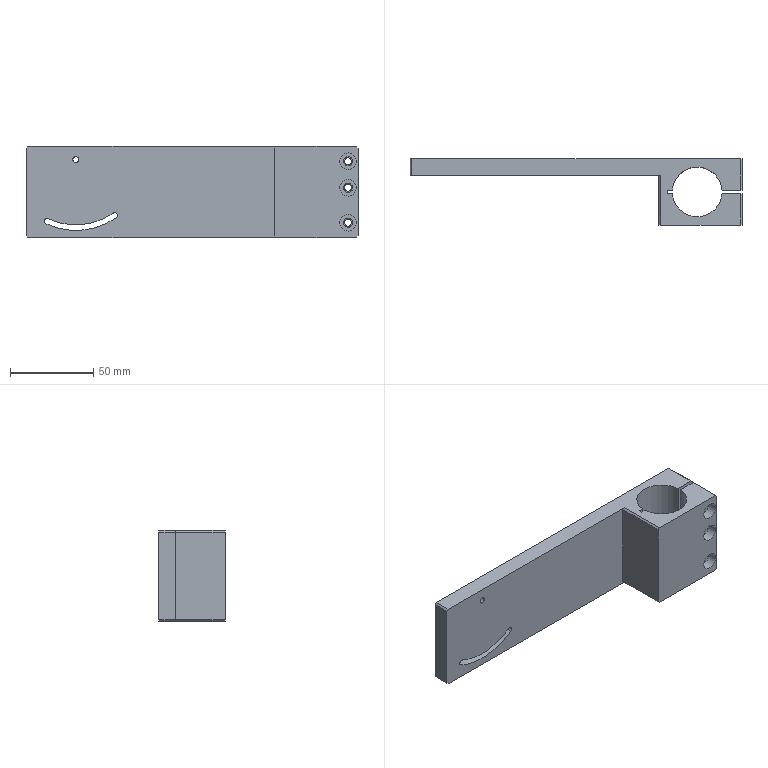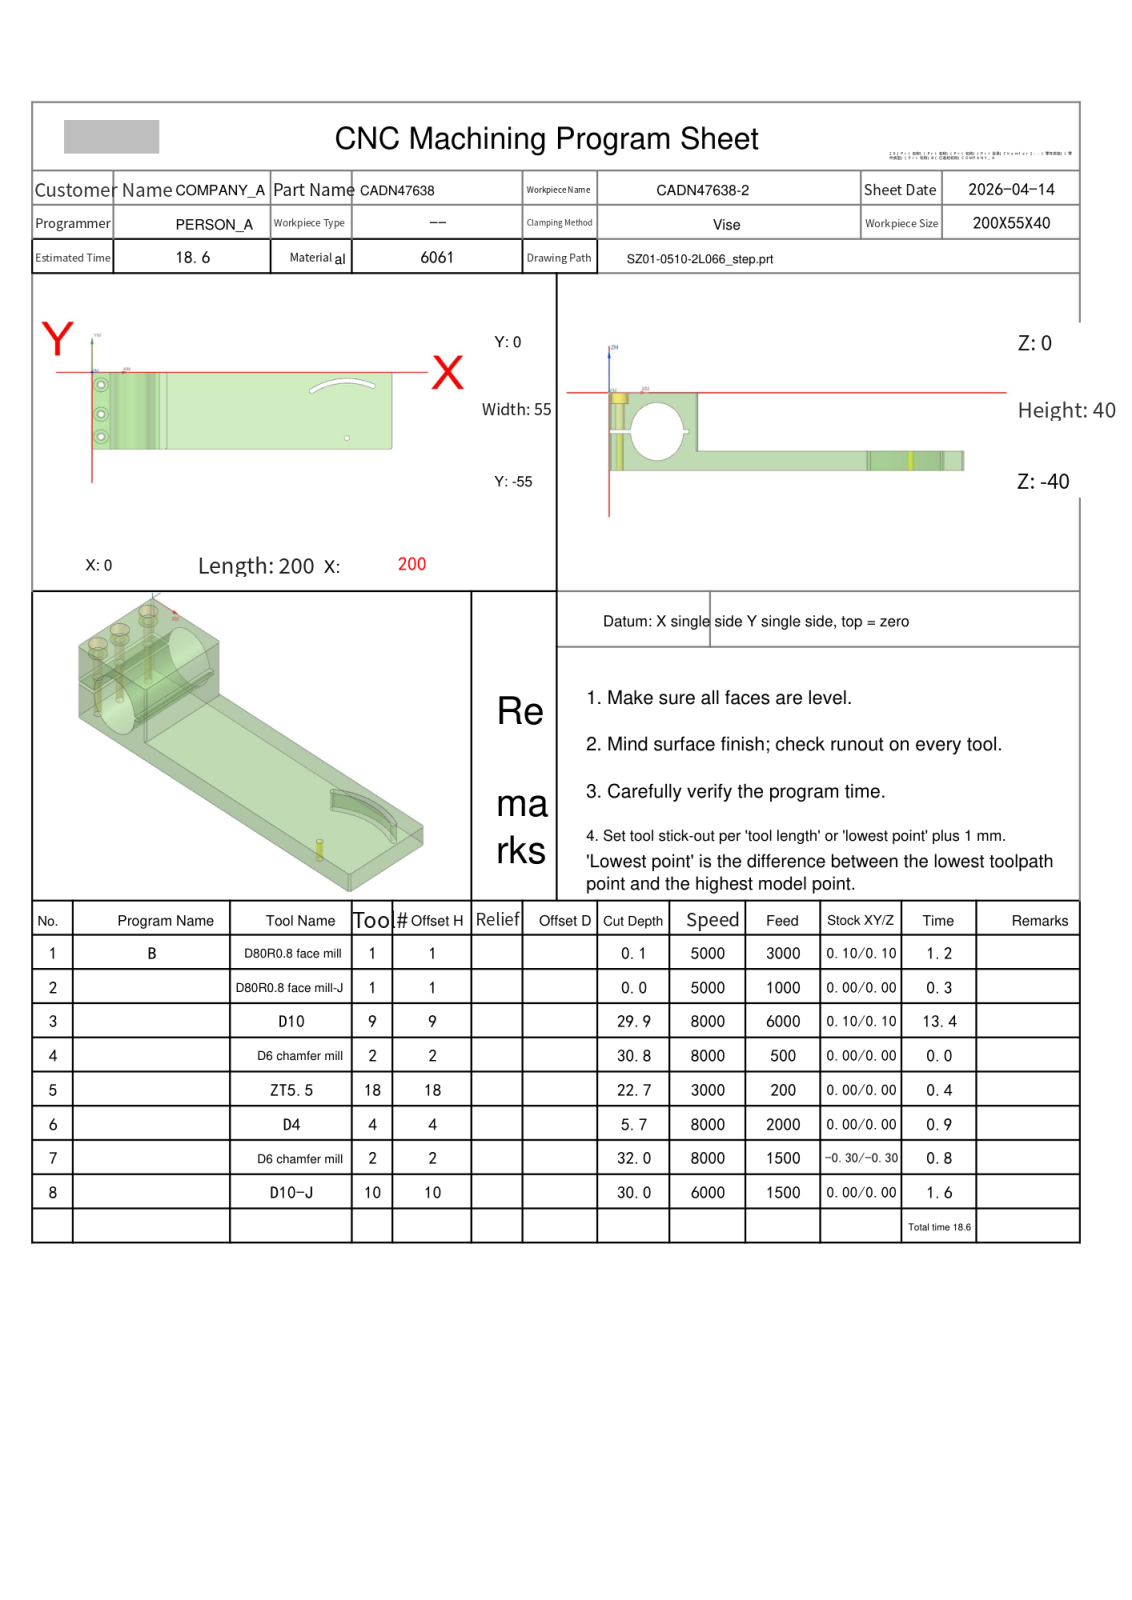NC program | NX | posted by the shop | part box 200 x 40 x 55 mm
Lines 7724 to 8619 of 8619:
N4 T02 M06
(D6 chamfer mill D=6. R=0. H=02 ce=0.00 di=0.10)
(MAX_Z=20. MIN_Z=-30.8 Time=0.04M)
G00 G90 G54 X170. Y-47. M03 S8000
G43 H02 Z20.
M08
G98 G81 X170. Y-47. Z-30.8 R-29. F500.
X6. Y-46. Z-.8 R1.
Y-30.
Y-9.
G80
G00 Z20.
G91 G28 Z0.0
M05
M09
G91 G28 Z0.0
M01
N5 T18 M06
(ZT5.5 D=5.5 DR_a=118 H=18)
(MAX_Z=20. MIN_Z=-22.65 Time=0.36M)
G00 G90 G54 X6. Y-46. M03 S3000
G43 H18 Z20.
M08
G98 G83 X6. Y-46. Z-22.652 R1. F200. Q2.
Y-30.
Y-9.
G80
G00 Z20.
G91 G28 Z0.0
M05
M09
G91 G28 Z0.0
M01
N6 T04 M06
(D4  D=4. R=0. H=04 ce=0.10 di=0.08)
(D.N=04 MAX_Z=20. MIN_Z=-5.7 Time=0.92M)
G00 G90 G54 X4.558 Y-32.526 M03 S8000
G43 H04 Z20.
M08
Z.8
G01 X4.688 Y-32.62 Z.792 F2000.
X5.582 Y-32.9 Z.743
X6.418 Z.699
X7.312 Y-32.62 Z.65
X8.072 Y-32.072 Z.601
X8.62 Y-31.312 Z.551
X8.9 Y-30.418 Z.502
Y-29.582 Z.458
X8.62 Y-28.688 Z.409
X8.072 Y-27.928 Z.36
X7.312 Y-27.38 Z.311
X6.418 Y-27.1 Z.262
X5.582 Z.218
X4.688 Y-27.38 Z.169
X3.928 Y-27.928 Z.12
X3.38 Y-28.688 Z.071
X3.1 Y-29.582 Z.022
Y-30. Z0.0
G03 X6. Y-32.9 Z-.074 I2.9 J0.0
X8.9 Y-30. Z-.148 I0.0 J2.9
X6. Y-27.1 Z-.223 I-2.9 J0.0
X3.1 Y-30. Z-.297 I0.0 J-2.9
X6. Y-32.9 Z-.371 I2.9 J0.0
X8.9 Y-30. Z-.445 I0.0 J2.9
X6. Y-27.1 Z-.519 I-2.9 J0.0
X3.1 Y-30. Z-.594 I0.0 J-2.9
X6. Y-32.9 Z-.668 I2.9 J0.0
X8.9 Y-30. Z-.742 I0.0 J2.9
X6. Y-27.1 Z-.816 I-2.9 J0.0
X3.1 Y-30. Z-.891 I0.0 J-2.9
X6. Y-32.9 Z-.965 I2.9 J0.0
X8.9 Y-30. Z-1.039 I0.0 J2.9
X6. Y-27.1 Z-1.113 I-2.9 J0.0
X3.1 Y-30. Z-1.187 I0.0 J-2.9
X6. Y-32.9 Z-1.262 I2.9 J0.0
X8.9 Y-30. Z-1.336 I0.0 J2.9
X6. Y-27.1 Z-1.41 I-2.9 J0.0
X3.1 Y-30. Z-1.484 I0.0 J-2.9
X6. Y-32.9 Z-1.558 I2.9 J0.0
X8.9 Y-30. Z-1.633 I0.0 J2.9
X6. Y-27.1 Z-1.707 I-2.9 J0.0
X3.1 Y-30. Z-1.781 I0.0 J-2.9
X6. Y-32.9 Z-1.855 I2.9 J0.0
X8.9 Y-30. Z-1.929 I0.0 J2.9
X6. Y-27.1 Z-2.004 I-2.9 J0.0
X3.1 Y-30. Z-2.078 I0.0 J-2.9
X6. Y-32.9 Z-2.152 I2.9 J0.0
X8.9 Y-30. Z-2.226 I0.0 J2.9
X6. Y-27.1 Z-2.301 I-2.9 J0.0
X3.1 Y-30. Z-2.375 I0.0 J-2.9
X6. Y-32.9 Z-2.449 I2.9 J0.0
X8.9 Y-30. Z-2.523 I0.0 J2.9
X6. Y-27.1 Z-2.597 I-2.9 J0.0
X3.1 Y-30. Z-2.672 I0.0 J-2.9
X6. Y-32.9 Z-2.746 I2.9 J0.0
X8.9 Y-30. Z-2.82 I0.0 J2.9
X6. Y-27.1 Z-2.894 I-2.9 J0.0
X3.1 Y-30. Z-2.968 I0.0 J-2.9
X6. Y-32.9 Z-3.043 I2.9 J0.0
X8.9 Y-30. Z-3.117 I0.0 J2.9
X6. Y-27.1 Z-3.191 I-2.9 J0.0
X3.1 Y-30. Z-3.265 I0.0 J-2.9
X6. Y-32.9 Z-3.339 I2.9 J0.0
X8.9 Y-30. Z-3.414 I0.0 J2.9
X6. Y-27.1 Z-3.488 I-2.9 J0.0
X3.1 Y-30. Z-3.562 I0.0 J-2.9
X6. Y-32.9 Z-3.636 I2.9 J0.0
X8.9 Y-30. Z-3.711 I0.0 J2.9
X6. Y-27.1 Z-3.785 I-2.9 J0.0
X3.1 Y-30. Z-3.859 I0.0 J-2.9
X6. Y-32.9 Z-3.933 I2.9 J0.0
X8.9 Y-30. Z-4.007 I0.0 J2.9
X6. Y-27.1 Z-4.082 I-2.9 J0.0
X3.1 Y-30. Z-4.156 I0.0 J-2.9
X6. Y-32.9 Z-4.23 I2.9 J0.0
X8.9 Y-30. Z-4.304 I0.0 J2.9
X6. Y-27.1 Z-4.378 I-2.9 J0.0
X3.1 Y-30. Z-4.453 I0.0 J-2.9
X6. Y-32.9 Z-4.527 I2.9 J0.0
X8.9 Y-30. Z-4.601 I0.0 J2.9
X6. Y-27.1 Z-4.675 I-2.9 J0.0
X3.1 Y-30. Z-4.749 I0.0 J-2.9
X6. Y-32.9 Z-4.824 I2.9 J0.0
X8.9 Y-30. Z-4.898 I0.0 J2.9
X6. Y-27.1 Z-4.972 I-2.9 J0.0
X3.1 Y-30. Z-5.046 I0.0 J-2.9
X6. Y-32.9 Z-5.121 I2.9 J0.0
X8.9 Y-30. Z-5.195 I0.0 J2.9
X6. Y-27.1 Z-5.269 I-2.9 J0.0
X3.1 Y-30. Z-5.343 I0.0 J-2.9
X6. Y-32.9 Z-5.417 I2.9 J0.0
X8.9 Y-30. Z-5.492 I0.0 J2.9
X6. Y-27.1 Z-5.566 I-2.9 J0.0
X3.1 Y-30. Z-5.64 I0.0 J-2.9
X6. Y-32.9 I2.9 J0.0
X8.9 Y-30. I0.0 J2.9
X6. Y-27.1 I-2.9 J0.0
X3.1 Y-30. I0.0 J-2.9
X3.128 Y-30.399 I2.9 J0.0
G01 Z-4.84
G00 Z20.
X4.558 Y-48.526
Z.8
G01 X4.688 Y-48.62 Z.792
X5.582 Y-48.9 Z.743
X6.418 Z.699
X7.312 Y-48.62 Z.65
X8.072 Y-48.072 Z.601
X8.62 Y-47.312 Z.551
X8.9 Y-46.418 Z.502
Y-45.582 Z.458
X8.62 Y-44.688 Z.409
X8.072 Y-43.928 Z.36
X7.312 Y-43.38 Z.311
X6.418 Y-43.1 Z.262
X5.582 Z.218
X4.688 Y-43.38 Z.169
X3.928 Y-43.928 Z.12
X3.38 Y-44.688 Z.071
X3.1 Y-45.582 Z.022
Y-46. Z0.0
G03 X6. Y-48.9 Z-.074 I2.9 J0.0
X8.9 Y-46. Z-.148 I0.0 J2.9
X6. Y-43.1 Z-.223 I-2.9 J0.0
X3.1 Y-46. Z-.297 I0.0 J-2.9
X6. Y-48.9 Z-.371 I2.9 J0.0
X8.9 Y-46. Z-.445 I0.0 J2.9
X6. Y-43.1 Z-.519 I-2.9 J0.0
X3.1 Y-46. Z-.594 I0.0 J-2.9
X6. Y-48.9 Z-.668 I2.9 J0.0
X8.9 Y-46. Z-.742 I0.0 J2.9
X6. Y-43.1 Z-.816 I-2.9 J0.0
X3.1 Y-46. Z-.891 I0.0 J-2.9
X6. Y-48.9 Z-.965 I2.9 J0.0
X8.9 Y-46. Z-1.039 I0.0 J2.9
X6. Y-43.1 Z-1.113 I-2.9 J0.0
X3.1 Y-46. Z-1.187 I0.0 J-2.9
X6. Y-48.9 Z-1.262 I2.9 J0.0
X8.9 Y-46. Z-1.336 I0.0 J2.9
X6. Y-43.1 Z-1.41 I-2.9 J0.0
X3.1 Y-46. Z-1.484 I0.0 J-2.9
X6. Y-48.9 Z-1.558 I2.9 J0.0
X8.9 Y-46. Z-1.633 I0.0 J2.9
X6. Y-43.1 Z-1.707 I-2.9 J0.0
X3.1 Y-46. Z-1.781 I0.0 J-2.9
X6. Y-48.9 Z-1.855 I2.9 J0.0
X8.9 Y-46. Z-1.929 I0.0 J2.9
X6. Y-43.1 Z-2.004 I-2.9 J0.0
X3.1 Y-46. Z-2.078 I0.0 J-2.9
X6. Y-48.9 Z-2.152 I2.9 J0.0
X8.9 Y-46. Z-2.226 I0.0 J2.9
X6. Y-43.1 Z-2.301 I-2.9 J0.0
X3.1 Y-46. Z-2.375 I0.0 J-2.9
X6. Y-48.9 Z-2.449 I2.9 J0.0
X8.9 Y-46. Z-2.523 I0.0 J2.9
X6. Y-43.1 Z-2.597 I-2.9 J0.0
X3.1 Y-46. Z-2.672 I0.0 J-2.9
X6. Y-48.9 Z-2.746 I2.9 J0.0
X8.9 Y-46. Z-2.82 I0.0 J2.9
X6. Y-43.1 Z-2.894 I-2.9 J0.0
X3.1 Y-46. Z-2.968 I0.0 J-2.9
X6. Y-48.9 Z-3.043 I2.9 J0.0
X8.9 Y-46. Z-3.117 I0.0 J2.9
X6. Y-43.1 Z-3.191 I-2.9 J0.0
X3.1 Y-46. Z-3.265 I0.0 J-2.9
X6. Y-48.9 Z-3.339 I2.9 J0.0
X8.9 Y-46. Z-3.414 I0.0 J2.9
X6. Y-43.1 Z-3.488 I-2.9 J0.0
X3.1 Y-46. Z-3.562 I0.0 J-2.9
X6. Y-48.9 Z-3.636 I2.9 J0.0
X8.9 Y-46. Z-3.711 I0.0 J2.9
X6. Y-43.1 Z-3.785 I-2.9 J0.0
X3.1 Y-46. Z-3.859 I0.0 J-2.9
X6. Y-48.9 Z-3.933 I2.9 J0.0
X8.9 Y-46. Z-4.007 I0.0 J2.9
X6. Y-43.1 Z-4.082 I-2.9 J0.0
X3.1 Y-46. Z-4.156 I0.0 J-2.9
X6. Y-48.9 Z-4.23 I2.9 J0.0
X8.9 Y-46. Z-4.304 I0.0 J2.9
X6. Y-43.1 Z-4.378 I-2.9 J0.0
X3.1 Y-46. Z-4.453 I0.0 J-2.9
X6. Y-48.9 Z-4.527 I2.9 J0.0
X8.9 Y-46. Z-4.601 I0.0 J2.9
X6. Y-43.1 Z-4.675 I-2.9 J0.0
X3.1 Y-46. Z-4.749 I0.0 J-2.9
X6. Y-48.9 Z-4.824 I2.9 J0.0
X8.9 Y-46. Z-4.898 I0.0 J2.9
X6. Y-43.1 Z-4.972 I-2.9 J0.0
X3.1 Y-46. Z-5.046 I0.0 J-2.9
X6. Y-48.9 Z-5.121 I2.9 J0.0
X8.9 Y-46. Z-5.195 I0.0 J2.9
X6. Y-43.1 Z-5.269 I-2.9 J0.0
X3.1 Y-46. Z-5.343 I0.0 J-2.9
X6. Y-48.9 Z-5.417 I2.9 J0.0
X8.9 Y-46. Z-5.492 I0.0 J2.9
X6. Y-43.1 Z-5.566 I-2.9 J0.0
X3.1 Y-46. Z-5.64 I0.0 J-2.9
X6. Y-48.9 I2.9 J0.0
X8.9 Y-46. I0.0 J2.9
X6. Y-43.1 I-2.9 J0.0
X3.1 Y-46. I0.0 J-2.9
X3.128 Y-46.399 I2.9 J0.0
G01 Z-4.84
G00 Z20.
X4.558 Y-11.526
Z.8
G01 X4.688 Y-11.62 Z.792
X5.582 Y-11.9 Z.743
X6.418 Z.699
X7.312 Y-11.62 Z.65
X8.072 Y-11.072 Z.601
X8.62 Y-10.312 Z.551
X8.9 Y-9.418 Z.502
Y-8.582 Z.458
X8.62 Y-7.688 Z.409
X8.072 Y-6.928 Z.36
X7.312 Y-6.38 Z.311
X6.418 Y-6.1 Z.262
X5.582 Z.218
X4.688 Y-6.38 Z.169
X3.928 Y-6.928 Z.12
X3.38 Y-7.688 Z.071
X3.1 Y-8.582 Z.022
Y-9. Z0.0
G03 X6. Y-11.9 Z-.074 I2.9 J0.0
X8.9 Y-9. Z-.148 I0.0 J2.9
X6. Y-6.1 Z-.223 I-2.9 J0.0
X3.1 Y-9. Z-.297 I0.0 J-2.9
X6. Y-11.9 Z-.371 I2.9 J0.0
X8.9 Y-9. Z-.445 I0.0 J2.9
X6. Y-6.1 Z-.519 I-2.9 J0.0
X3.1 Y-9. Z-.594 I0.0 J-2.9
X6. Y-11.9 Z-.668 I2.9 J0.0
X8.9 Y-9. Z-.742 I0.0 J2.9
X6. Y-6.1 Z-.816 I-2.9 J0.0
X3.1 Y-9. Z-.891 I0.0 J-2.9
X6. Y-11.9 Z-.965 I2.9 J0.0
X8.9 Y-9. Z-1.039 I0.0 J2.9
X6. Y-6.1 Z-1.113 I-2.9 J0.0
X3.1 Y-9. Z-1.187 I0.0 J-2.9
X6. Y-11.9 Z-1.262 I2.9 J0.0
X8.9 Y-9. Z-1.336 I0.0 J2.9
X6. Y-6.1 Z-1.41 I-2.9 J0.0
X3.1 Y-9. Z-1.484 I0.0 J-2.9
X6. Y-11.9 Z-1.558 I2.9 J0.0
X8.9 Y-9. Z-1.633 I0.0 J2.9
X6. Y-6.1 Z-1.707 I-2.9 J0.0
X3.1 Y-9. Z-1.781 I0.0 J-2.9
X6. Y-11.9 Z-1.855 I2.9 J0.0
X8.9 Y-9. Z-1.929 I0.0 J2.9
X6. Y-6.1 Z-2.004 I-2.9 J0.0
X3.1 Y-9. Z-2.078 I0.0 J-2.9
X6. Y-11.9 Z-2.152 I2.9 J0.0
X8.9 Y-9. Z-2.226 I0.0 J2.9
X6. Y-6.1 Z-2.301 I-2.9 J0.0
X3.1 Y-9. Z-2.375 I0.0 J-2.9
X6. Y-11.9 Z-2.449 I2.9 J0.0
X8.9 Y-9. Z-2.523 I0.0 J2.9
X6. Y-6.1 Z-2.597 I-2.9 J0.0
X3.1 Y-9. Z-2.672 I0.0 J-2.9
X6. Y-11.9 Z-2.746 I2.9 J0.0
X8.9 Y-9. Z-2.82 I0.0 J2.9
X6. Y-6.1 Z-2.894 I-2.9 J0.0
X3.1 Y-9. Z-2.968 I0.0 J-2.9
X6. Y-11.9 Z-3.043 I2.9 J0.0
X8.9 Y-9. Z-3.117 I0.0 J2.9
X6. Y-6.1 Z-3.191 I-2.9 J0.0
X3.1 Y-9. Z-3.265 I0.0 J-2.9
X6. Y-11.9 Z-3.339 I2.9 J0.0
X8.9 Y-9. Z-3.414 I0.0 J2.9
X6. Y-6.1 Z-3.488 I-2.9 J0.0
X3.1 Y-9. Z-3.562 I0.0 J-2.9
X6. Y-11.9 Z-3.636 I2.9 J0.0
X8.9 Y-9. Z-3.711 I0.0 J2.9
X6. Y-6.1 Z-3.785 I-2.9 J0.0
X3.1 Y-9. Z-3.859 I0.0 J-2.9
X6. Y-11.9 Z-3.933 I2.9 J0.0
X8.9 Y-9. Z-4.007 I0.0 J2.9
X6. Y-6.1 Z-4.082 I-2.9 J0.0
X3.1 Y-9. Z-4.156 I0.0 J-2.9
X6. Y-11.9 Z-4.23 I2.9 J0.0
X8.9 Y-9. Z-4.304 I0.0 J2.9
X6. Y-6.1 Z-4.378 I-2.9 J0.0
X3.1 Y-9. Z-4.453 I0.0 J-2.9
X6. Y-11.9 Z-4.527 I2.9 J0.0
X8.9 Y-9. Z-4.601 I0.0 J2.9
X6. Y-6.1 Z-4.675 I-2.9 J0.0
X3.1 Y-9. Z-4.749 I0.0 J-2.9
X6. Y-11.9 Z-4.824 I2.9 J0.0
X8.9 Y-9. Z-4.898 I0.0 J2.9
X6. Y-6.1 Z-4.972 I-2.9 J0.0
X3.1 Y-9. Z-5.046 I0.0 J-2.9
X6. Y-11.9 Z-5.121 I2.9 J0.0
X8.9 Y-9. Z-5.195 I0.0 J2.9
X6. Y-6.1 Z-5.269 I-2.9 J0.0
X3.1 Y-9. Z-5.343 I0.0 J-2.9
X6. Y-11.9 Z-5.417 I2.9 J0.0
X8.9 Y-9. Z-5.492 I0.0 J2.9
X6. Y-6.1 Z-5.566 I-2.9 J0.0
X3.1 Y-9. Z-5.64 I0.0 J-2.9
X6. Y-11.9 I2.9 J0.0
X8.9 Y-9. I0.0 J2.9
X6. Y-6.1 I-2.9 J0.0
X3.1 Y-9. I0.0 J-2.9
X3.128 Y-9.399 I2.9 J0.0
G01 Z-4.84
G00 Z20.
G00 G90 X8.953 Y-46.254 M03 S8000
Z20.
Z.5
G01 X8.965 Y-46.172 Z.496 F800.
Y-45.828 Z.478
X8.898 Y-45.353 Z.452
X8.757 Y-44.895 Z.427
X8.543 Y-44.466 Z.402
X8.263 Y-44.076 Z.377
X7.924 Y-43.737 Z.352
X7.534 Y-43.457 Z.327
X7.105 Y-43.243 Z.302
X6.647 Y-43.102 Z.277
X6.172 Y-43.035 Z.251
X5.828 Z.233
X5.439 Y-43.084 Z.213
X5.061 Y-43.183 Z.192
X4.699 Y-43.33 Z.172
X4.359 Y-43.525 Z.151
X4.083 Y-43.731 Z.133
X3.747 Y-44.066 Z.108
X3.467 Y-44.449 Z.084
X3.253 Y-44.872 Z.059
X3.108 Y-45.323 Z.034
X3.037 Y-45.792 Z.009
X3.035 Y-45.965 Z0.0
G41 D04
X3. Y-46.
G03 X6. Y-49. Z-.475 I3. J0.0
X9. Y-46. Z-.95 I0.0 J3.
X6. Y-43. Z-1.425 I-3. J0.0
X4.2 Y-43.6 Z-1.62 I0.0 J-3.
X3. Y-46. Z-1.9 I1.8 J-2.4
X6. Y-49. Z-2.375 I3. J0.0
X9. Y-46. Z-2.85 I0.0 J3.
X6. Y-43. Z-3.325 I-3. J0.0
X4.2 Y-43.6 Z-3.52 I0.0 J-3.
X3. Y-46. Z-3.8 I1.8 J-2.4
X6. Y-49. Z-4.275 I3. J0.0
X9. Y-46. Z-4.75 I0.0 J3.
X6. Y-43. Z-5.225 I-3. J0.0
X4.2 Y-43.6 Z-5.42 I0.0 J-3.
X3. Y-46. Z-5.7 I1.8 J-2.4
X6. Y-49. I3. J0.0
X9. Y-46. I0.0 J3.
X6. Y-43. I-3. J0.0
X3. Y-46. I0.0 J-3.
X3.027 Y-46.399 I3. J0.0
G01 X3.033 Y-46.426
X3.055 Y-46.443
X3.083 Y-46.442
G40 X3.132 Y-46.435
Z-4.7
G00 Z20.
X8.953 Y-30.255
Z.5
G01 X8.965 Y-30.172 Z.496
Y-29.828 Z.478
X8.898 Y-29.353 Z.452
X8.757 Y-28.895 Z.427
X8.543 Y-28.466 Z.402
X8.263 Y-28.076 Z.377
X7.924 Y-27.737 Z.352
X7.534 Y-27.457 Z.327
X7.105 Y-27.243 Z.302
X6.647 Y-27.102 Z.277
X6.172 Y-27.035 Z.251
X5.828 Z.233
X5.357 Y-27.101 Z.208
X4.902 Y-27.241 Z.184
X4.476 Y-27.451 Z.159
X4.088 Y-27.727 Z.134
X3.75 Y-28.061 Z.109
X3.47 Y-28.445 Z.084
X3.254 Y-28.869 Z.059
X3.109 Y-29.322 Z.034
X3.037 Y-29.792 Z.009
X3.035 Y-29.965 Z0.0
G41 D04
X3. Y-30.
G03 X6. Y-33. Z-.475 I3. J0.0
X9. Y-30. Z-.95 I0.0 J3.
X6. Y-27. Z-1.425 I-3. J0.0
X3. Y-30. Z-1.9 I0.0 J-3.
X6. Y-33. Z-2.375 I3. J0.0
X9. Y-30. Z-2.85 I0.0 J3.
X6. Y-27. Z-3.325 I-3. J0.0
X3. Y-30. Z-3.8 I0.0 J-3.
X6. Y-33. Z-4.275 I3. J0.0
X9. Y-30. Z-4.75 I0.0 J3.
X6. Y-27. Z-5.225 I-3. J0.0
X3. Y-30. Z-5.7 I0.0 J-3.
X6. Y-33. I3. J0.0
X9. Y-30. I0.0 J3.
X6. Y-27. I-3. J0.0
X3. Y-30. I0.0 J-3.
X3.027 Y-30.399 I3. J0.0
G01 X3.033 Y-30.426
X3.055 Y-30.443
X3.083 Y-30.442
G40 X3.132 Y-30.435
Z-4.7
G00 Z20.
X8.953 Y-9.254
Z.5
G01 X8.965 Y-9.172 Z.496
Y-8.828 Z.478
X8.906 Y-8.389 Z.454
X8.783 Y-7.964 Z.431
X8.598 Y-7.561 Z.408
X8.355 Y-7.191 Z.385
X8.13 Y-6.931 Z.367
X7.801 Y-6.638 Z.344
X7.432 Y-6.398 Z.321
X7.032 Y-6.215 Z.298
X6.609 Y-6.093 Z.274
X6.172 Y-6.035 Z.251
X5.828 Z.233
X5.357 Y-6.101 Z.208
X4.902 Y-6.241 Z.184
X4.476 Y-6.451 Z.159
X4.088 Y-6.727 Z.134
X3.75 Y-7.061 Z.109
X3.47 Y-7.445 Z.084
X3.254 Y-7.869 Z.059
X3.109 Y-8.322 Z.034
X3.037 Y-8.792 Z.009
X3.035 Y-8.965 Z0.0
G41 D04
X3. Y-9.
G03 X6. Y-12. Z-.475 I3. J0.0
X9. Y-9. Z-.95 I0.0 J3.
X8.269 Y-7.038 Z-1.166 I-3. J0.0
X6. Y-6. Z-1.425 I-2.269 J-1.962
X3. Y-9. Z-1.9 I0.0 J-3.
X6. Y-12. Z-2.375 I3. J0.0
X9. Y-9. Z-2.85 I0.0 J3.
X8.269 Y-7.038 Z-3.066 I-3. J0.0
X6. Y-6. Z-3.325 I-2.269 J-1.962
X3. Y-9. Z-3.8 I0.0 J-3.
X6. Y-12. Z-4.275 I3. J0.0
X9. Y-9. Z-4.75 I0.0 J3.
X8.269 Y-7.038 Z-4.966 I-3. J0.0
X6. Y-6. Z-5.225 I-2.269 J-1.962
X3. Y-9. Z-5.7 I0.0 J-3.
X6. Y-12. I3. J0.0
X9. Y-9. I0.0 J3.
X6. Y-6. I-3. J0.0
X3. Y-9. I0.0 J-3.
X3.027 Y-9.399 I3. J0.0
G01 X3.033 Y-9.426
X3.055 Y-9.443
X3.083 Y-9.442
G40 X3.132 Y-9.435
Z-4.7
G00 Z20.
G91 G28 Z0.0
M05
M09
G91 G28 Z0.0
M01
N7 T02 M06
(D6 chamfer mill D=6. R=0. H=02 ce=0.00 di=0.00)
(MAX_Z=20. MIN_Z=-32.05 Time=0.77M)
G00 G90 G54 X170. Y-47. M03 S8000
G43 H02 Z20.
M08
G98 G81 X170. Y-47. Z-32.05 R-27. F500.
G80
G00 Z20.
G00 G90 X9. Y-45.219 M03 S8000
Z20.
Z-.7
G01 Z-1.2 F800.
Y-44.9
G03 X6. Y-41.9 I-3. J0.0
X1.9 Y-46. I0.0 J-4.1
X6. Y-50.1 I4.1 J0.0
X10.1 Y-46. I0.0 J4.1
X6. Y-41.9 I-4.1 J0.0
X3. Y-44.9 I0.0 J-3.
G01 Y-45.219
Z-.7
G00 Z20.
X9. Y-29.219
Z-.7
G01 Z-1.2
Y-28.9
G03 X6. Y-25.9 I-3. J0.0
X1.9 Y-30. I0.0 J-4.1
X6. Y-34.1 I4.1 J0.0
X10.1 Y-30. I0.0 J4.1
X6. Y-25.9 I-4.1 J0.0
X3. Y-28.9 I0.0 J-3.
G01 Y-29.219
Z-.7
G00 Z20.
X9. Y-8.219
Z-.7
G01 Z-1.2
Y-7.9
G03 X6. Y-4.9 I-3. J0.0
X1.9 Y-9. I0.0 J-4.1
X6. Y-13.1 I4.1 J0.0
X10.1 Y-9. I0.0 J4.1
X6. Y-4.9 I-4.1 J0.0
X3. Y-7.9 I0.0 J-3.
G01 Y-8.219
Z-.7
G00 Z20.
G00 G90 X-1.227 Y-27.886 M03 S6500
Z20.
Z.172
G01 Z-1.2 F1500.
G03 X-1.027 Y-27.6 I-1.532 J1.286
G01 X-.997 Y-27.554
X-1. Y-27.5
Y-1.
X-.966 Y-.741
X-.866 Y-.5
X-.707 Y-.293
X.293 Y.707
X.5 Y.866
X.741 Y.966
X1. Y1.
X49.
X49.259 Y.966
X49.5 Y.866
X49.707 Y.707
X50.707 Y-.293
X50.866 Y-.5
X50.966 Y-.741
X51. Y-1.
Y-54.
X50.966 Y-54.259
X50.866 Y-54.5
X50.707 Y-54.707
X49.707 Y-55.707
X49.5 Y-55.866
X49.259 Y-55.966
X49. Y-56.
X1.
X.741 Y-55.966
X.5 Y-55.866
X.293 Y-55.707
X-.707 Y-54.707
X-.866 Y-54.5
X-.966 Y-54.259
X-1. Y-54.
Y-27.5
X-.997 Y-27.446
X-1.027 Y-27.4
G03 X-1.227 Y-27.114 I-1.732 J-1.
G01 Z.172
G00 Z10.
X6.4 Y-42.201
Z.225
G01 Z-1.2
G03 X6.102 Y-42.02 I-1.183 J-1.613
G01 X6.054 Y-41.994
X6. Y-42.
G03 X2. Y-46. I0.0 J-4.
X6. Y-50. I4. J0.0
X10. Y-46. I0.0 J4.
X6. Y-42. I-4. J0.0
G01 X5.946 Y-41.994
X5.898 Y-42.02
G03 X5.6 Y-42.201 I.885 J-1.794
G01 Z.225
G00 Z10.
X6.4 Y-26.201
Z.225
G01 Z-1.2
G03 X6.102 Y-26.02 I-1.183 J-1.613
G01 X6.054 Y-25.994
X6. Y-26.
G03 X2. Y-30. I0.0 J-4.
X6. Y-34. I4. J0.0
X10. Y-30. I0.0 J4.
X6. Y-26. I-4. J0.0
G01 X5.946 Y-25.994
X5.898 Y-26.02
G03 X5.6 Y-26.201 I.885 J-1.794
G01 Z.225
G00 Z10.
X6.4 Y-5.201
Z.225
G01 Z-1.2
G03 X6.102 Y-5.02 I-1.183 J-1.613
G01 X6.054 Y-4.994
X6. Y-5.
G03 X2. Y-9. I0.0 J-4.
X6. Y-13. I4. J0.0
X10. Y-9. I0.0 J4.
X6. Y-5. I-4. J0.0
G01 X5.946 Y-4.994
X5.898 Y-5.02
G03 X5.6 Y-5.201 I.885 J-1.794
G01 Z.225
G00 Z10.
X52.396 Y1.113
Z-1.796
G01 Z-31.199
X52.46 Y1.052
X52.539 Y1.013
X52.56 Y.994
X52.589 Y1.
X199.
X199.259 Y.966
X199.5 Y.866
X199.707 Y.707
X200.707 Y-.293
X200.866 Y-.5
X200.966 Y-.741
X201. Y-1.
Y-54.
X200.966 Y-54.259
X200.866 Y-54.5
X200.707 Y-54.707
X199.707 Y-55.707
X199.5 Y-55.866
X199.259 Y-55.966
X199. Y-56.
X52.589
X52.56 Y-55.994
X52.539 Y-56.013
X52.46 Y-56.052
X52.396 Y-56.113
Z-1.796
G00 Z10.
X187.706 Y-9.703
Z-29.825
G01 Z-31.199
G03 X187.645 Y-9.36 I-1.992 J-.174
G01 X187.634 Y-9.307
X187.594 Y-9.27
G03 X170. Y-5.37 I-17.594 J-37.73
X146.122 Y-12.899 I0.0 J-41.63
X145.845 Y-13.431 I.373 J-.532
X146.104 Y-13.95 I.65 J0.0
G01 X146.283 Y-14.046
X146.483 Y-14.081
X146.685 Y-14.053
X146.868 Y-13.964
G02 X170. Y-6.67 I23.132 J-33.036
X187.044 Y-10.449 I0.0 J-40.33
G03 X187.319 Y-10.51 I.275 J.589
X187.964 Y-9.939 I0.0 J.65
G01 X187.957 Y-9.735
X187.887 Y-9.544
X187.762 Y-9.384
X187.594 Y-9.27
X187.55 Y-9.238
X187.496 Y-9.237
X187.356 Y-9.232
G03 X187.147 Y-9.243 I0.0 J-2.
G01 Z-29.756
G00 Z10.
X170.412 Y-46.424
Z-29.637
G01 Z-31.199
G03 X170.103 Y-46.264 I-1.075 J-1.687
G01 X170.054 Y-46.24
X170. Y-46.25
G03 X169.25 Y-47. I0.0 J-.75
X170. Y-47.75 I.75 J0.0
X170.75 Y-47. I0.0 J.75
X170.194 Y-46.276 I-.75 J0.0
G01 X170. Y-46.25
X169.946 Y-46.24
X169.897 Y-46.264
G03 X169.588 Y-46.424 I.765 J-1.848
G01 Z-29.637
G00 Z20.
G91 G28 Z0.0
M05
M09
G91 G28 Z0.0
M01
N8 T10 M06
(D10-J  D=10. R=0. H=10 ce=0.40 di=0.00)
(D.N=10 MAX_Z=14.8 MIN_Z=-30. Time=1.61M)
G00 G90 G54 X202.036 Y6.752 M03 S6000
G43 H10 Z14.8
M08
Z-28.5
G01 Z-30. F1500.
G03 X201. Y5. I.964 J-1.752
G01 Y-59.1
G02 X200.1 Y-60. I-.9 J0.0
G01 X197.147
G02 X196.147 Y-59. I0.0 J1.
G01 Y4.1
G03 X195.247 Y5. I-.9 J0.0
G01 X192.293
G03 X191.293 Y4. I0.0 J-1.
G01 Y-59.1
G02 X190.393 Y-60. I-.9 J0.0
G01 X187.44
G02 X186.44 Y-59. I0.0 J1.
G01 Y4.1
G03 X185.54 Y5. I-.9 J0.0
G01 X182.587
G03 X181.587 Y4. I0.0 J-1.
G01 Y-59.1
G02 X180.687 Y-60. I-.9 J0.0
G01 X177.733
G02 X176.733 Y-59. I0.0 J1.
G01 Y4.1
G03 X175.833 Y5. I-.9 J0.0
G01 X172.88
G03 X171.88 Y4. I0.0 J-1.
G01 Y-59.1
G02 X170.98 Y-60. I-.9 J0.0
G01 X168.027
G02 X167.027 Y-59. I0.0 J1.
G01 Y4.1
G03 X166.127 Y5. I-.9 J0.0
G01 X163.173
G03 X162.173 Y4. I0.0 J-1.
G01 Y-59.1
G02 X161.273 Y-60. I-.9 J0.0
G01 X158.32
G02 X157.32 Y-59. I0.0 J1.
G01 Y4.1
G03 X156.42 Y5. I-.9 J0.0
G01 X153.467
G03 X152.467 Y4. I0.0 J-1.
G01 Y-59.1
G02 X151.567 Y-60. I-.9 J0.0
G01 X148.613
G02 X147.613 Y-59. I0.0 J1.
G01 Y4.1
G03 X146.713 Y5. I-.9 J0.0
G01 X143.76
G03 X142.76 Y4. I0.0 J-1.
G01 Y-59.1
G02 X141.86 Y-60. I-.9 J0.0
G01 X138.907
G02 X137.907 Y-59. I0.0 J1.
G01 Y4.1
G03 X137.007 Y5. I-.9 J0.0
G01 X134.053
G03 X133.053 Y4. I0.0 J-1.
G01 Y-59.1
G02 X132.153 Y-60. I-.9 J0.0
G01 X129.2
G02 X128.2 Y-59. I0.0 J1.
G01 Y4.1
G03 X127.3 Y5. I-.9 J0.0
G01 X124.347
G03 X123.347 Y4. I0.0 J-1.
G01 Y-59.1
G02 X122.447 Y-60. I-.9 J0.0
G01 X119.493
G02 X118.493 Y-59. I0.0 J1.
G01 Y4.1
G03 X117.593 Y5. I-.9 J0.0
G01 X114.64
G03 X113.64 Y4. I0.0 J-1.
G01 Y-59.1
G02 X112.74 Y-60. I-.9 J0.0
G01 X109.787
G02 X108.787 Y-59. I0.0 J1.
G01 Y4.1
G03 X107.887 Y5. I-.9 J0.0
G01 X104.933
G03 X103.933 Y4. I0.0 J-1.
G01 Y-59.1
G02 X103.033 Y-60. I-.9 J0.0
G01 X100.08
G02 X99.08 Y-59. I0.0 J1.
G01 Y4.1
G03 X98.18 Y5. I-.9 J0.0
G01 X95.227
G03 X94.227 Y4. I0.0 J-1.
G01 Y-59.1
G02 X93.327 Y-60. I-.9 J0.0
G01 X90.373
G02 X89.373 Y-59. I0.0 J1.
G01 Y4.1
G03 X88.473 Y5. I-.9 J0.0
G01 X85.52
G03 X84.52 Y4. I0.0 J-1.
G01 Y-59.1
G02 X83.62 Y-60. I-.9 J0.0
G01 X80.667
G02 X79.667 Y-59. I0.0 J1.
G01 Y4.1
G03 X78.767 Y5. I-.9 J0.0
G01 X75.813
G03 X74.813 Y4. I0.0 J-1.
G01 Y-59.1
G02 X73.913 Y-60. I-.9 J0.0
G01 X70.96
G02 X69.96 Y-59. I0.0 J1.
G01 Y4.1
G03 X69.06 Y5. I-.9 J0.0
G01 X66.107
G03 X65.107 Y4. I0.0 J-1.
G01 Y-59.1
G02 X64.207 Y-60. I-.9 J0.0
G01 X61.253
G02 X60.253 Y-59. I0.0 J1.
G01 Y4.1
G03 X59.353 Y5. I-.9 J0.0
G01 X56.4
G03 X55.4 Y4. I0.0 J-1.
G01 Y-60.
G03 X57.399 Y-62. I2. J0.0
G01 Z-28.5
G00 Z14.8
G00 G90 X50.632 Y7.191 M03 S6000
Z14.8
Z-14.
G01 Z-15. F1000.
G41 D10
X50.573 Y7.
G03 X50.485 Y6.414 I1.912 J-.586
X51.071 Y5. I2. J0.0
G01 X55. Y1.071
Y-56.071
X51.071 Y-60.
G03 X50.485 Y-61.414 I1.414 J-1.414
X50.573 Y-62. I2. J0.0
G01 G40 X50.632 Y-62.191
Z-14.
G00 Z14.8
Y7.191
Z-29.
G01 Z-30.
G41 D10
X50.573 Y7.
G03 X50.485 Y6.414 I1.912 J-.586
X51.071 Y5. I2. J0.0
G01 X55. Y1.071
Y-56.071
X51.071 Y-60.
G03 X50.485 Y-61.414 I1.414 J-1.414
X50.573 Y-62. I2. J0.0
G01 G40 X50.632 Y-62.191
Z-29.
G00 Z14.8
M05
M09
G91 G28 Z0.0
G91 G28 Y0.0
M30
%